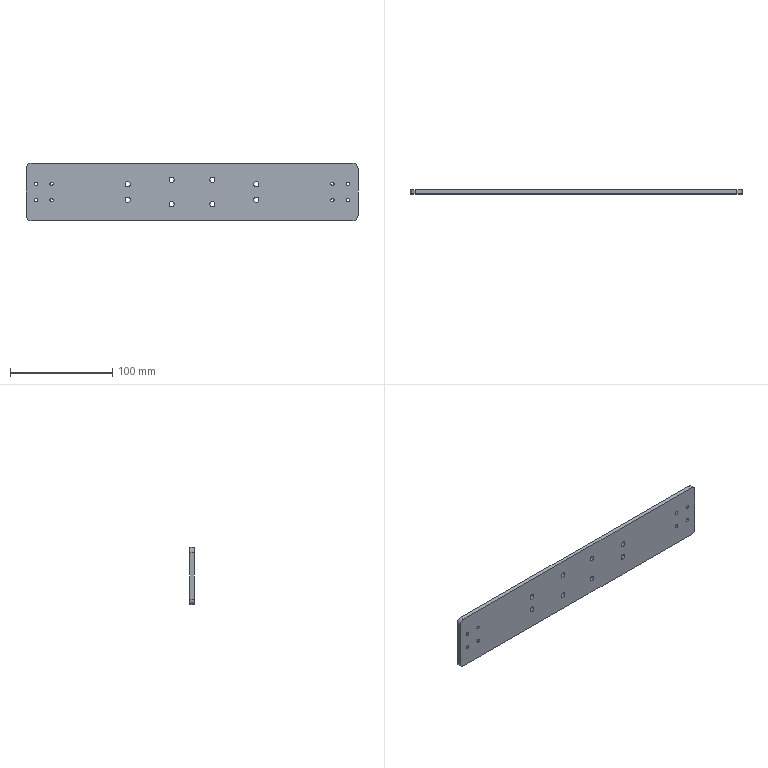Part | SolidWorks | features BaseBody 1 | 1 solid | 42 faces | box 325 x 4 x 56 mm | volume 71803 mm3 | cylinder 36 | plane 6 | commonest cylinder face diameters 3.2 x16 5 x8 5.2 x8 10 x4
STEP:
#1=CARTESIAN_POINT('',(63.,4.,10.1));
#2=VERTEX_POINT('',#1);
#3=CARTESIAN_POINT('',(63.,4.,4.9));
#4=VERTEX_POINT('',#3);
#5=CARTESIAN_POINT('',(63.,4.,7.5));
#6=DIRECTION('',(0.,-1.,0.));
#7=DIRECTION('',(0.,0.,-1.));
#8=AXIS2_PLACEMENT_3D('',#5,#6,#7);
#9=CIRCLE('',#8,2.6);
#10=EDGE_CURVE('',#2,#4,#9,.T.);
#11=ORIENTED_EDGE('',*,*,#10,.F.);
#12=CARTESIAN_POINT('',(63.,0.,10.1));
#13=VERTEX_POINT('',#12);
#14=CARTESIAN_POINT('',(63.,4.,10.1));
#15=DIRECTION('',(0.,-1.,0.));
#16=VECTOR('',#15,1000.);
#17=LINE('',#14,#16);
#18=EDGE_CURVE('',#2,#13,#17,.T.);
#19=ORIENTED_EDGE('',*,*,#18,.T.);
#20=CARTESIAN_POINT('',(63.,0.,4.9));
#21=VERTEX_POINT('',#20);
#22=CARTESIAN_POINT('',(63.,0.,7.5));
#23=DIRECTION('',(0.,-1.,0.));
#24=DIRECTION('',(0.,0.,-1.));
#25=AXIS2_PLACEMENT_3D('',#22,#23,#24);
#26=CIRCLE('',#25,2.6);
#27=EDGE_CURVE('',#13,#21,#26,.T.);
#28=ORIENTED_EDGE('',*,*,#27,.T.);
#29=CARTESIAN_POINT('',(63.,4.,4.9));
#30=DIRECTION('',(0.,-1.,0.));
#31=VECTOR('',#30,1000.);
#32=LINE('',#29,#31);
#33=EDGE_CURVE('',#4,#21,#32,.T.);
#34=ORIENTED_EDGE('',*,*,#33,.F.);
#35=EDGE_LOOP('',(#11,#19,#28,#34));
#36=FACE_OUTER_BOUND('',#35,.T.);
#37=CARTESIAN_POINT('',(63.,4.,7.5));
#38=DIRECTION('',(0.,-1.,0.));
#39=DIRECTION('',(0.,0.,-1.));
#40=AXIS2_PLACEMENT_3D('',#37,#38,#39);
#41=CYLINDRICAL_SURFACE('',#40,2.6);
#42=ADVANCED_FACE('',(#36),#41,.F.);
#43=CARTESIAN_POINT('',(63.,4.,-4.9));
#44=VERTEX_POINT('',#43);
#45=CARTESIAN_POINT('',(63.,4.,-10.1));
#46=VERTEX_POINT('',#45);
#47=CARTESIAN_POINT('',(63.,4.,-7.5));
#48=DIRECTION('',(0.,-1.,0.));
#49=DIRECTION('',(0.,0.,-1.));
#50=AXIS2_PLACEMENT_3D('',#47,#48,#49);
#51=CIRCLE('',#50,2.6);
#52=EDGE_CURVE('',#44,#46,#51,.T.);
#53=ORIENTED_EDGE('',*,*,#52,.F.);
#54=CARTESIAN_POINT('',(63.,0.,-4.9));
#55=VERTEX_POINT('',#54);
#56=CARTESIAN_POINT('',(63.,4.,-4.9));
#57=DIRECTION('',(0.,-1.,0.));
#58=VECTOR('',#57,1000.);
#59=LINE('',#56,#58);
#60=EDGE_CURVE('',#44,#55,#59,.T.);
#61=ORIENTED_EDGE('',*,*,#60,.T.);
#62=CARTESIAN_POINT('',(63.,0.,-10.1));
#63=VERTEX_POINT('',#62);
#64=CARTESIAN_POINT('',(63.,0.,-7.5));
#65=DIRECTION('',(0.,-1.,0.));
#66=DIRECTION('',(0.,0.,-1.));
#67=AXIS2_PLACEMENT_3D('',#64,#65,#66);
#68=CIRCLE('',#67,2.6);
#69=EDGE_CURVE('',#55,#63,#68,.T.);
#70=ORIENTED_EDGE('',*,*,#69,.T.);
#71=CARTESIAN_POINT('',(63.,4.,-10.1));
#72=DIRECTION('',(0.,-1.,0.));
#73=VECTOR('',#72,1000.);
#74=LINE('',#71,#73);
#75=EDGE_CURVE('',#46,#63,#74,.T.);
#76=ORIENTED_EDGE('',*,*,#75,.F.);
#77=EDGE_LOOP('',(#53,#61,#70,#76));
#78=FACE_OUTER_BOUND('',#77,.T.);
#79=CARTESIAN_POINT('',(63.,4.,-7.5));
#80=DIRECTION('',(0.,-1.,0.));
#81=DIRECTION('',(0.,0.,-1.));
#82=AXIS2_PLACEMENT_3D('',#79,#80,#81);
#83=CYLINDRICAL_SURFACE('',#82,2.6);
#84=ADVANCED_FACE('',(#78),#83,.F.);
#85=CARTESIAN_POINT('',(-63.,4.,-4.9));
#86=VERTEX_POINT('',#85);
#87=CARTESIAN_POINT('',(-63.,4.,-10.1));
#88=VERTEX_POINT('',#87);
#89=CARTESIAN_POINT('',(-63.,4.,-7.5));
#90=DIRECTION('',(0.,-1.,0.));
#91=DIRECTION('',(0.,0.,-1.));
#92=AXIS2_PLACEMENT_3D('',#89,#90,#91);
#93=CIRCLE('',#92,2.6);
#94=EDGE_CURVE('',#86,#88,#93,.T.);
#95=ORIENTED_EDGE('',*,*,#94,.F.);
#96=CARTESIAN_POINT('',(-63.,0.,-4.9));
#97=VERTEX_POINT('',#96);
#98=CARTESIAN_POINT('',(-63.,4.,-4.9));
#99=DIRECTION('',(0.,-1.,0.));
#100=VECTOR('',#99,1000.);
#101=LINE('',#98,#100);
#102=EDGE_CURVE('',#86,#97,#101,.T.);
#103=ORIENTED_EDGE('',*,*,#102,.T.);
#104=CARTESIAN_POINT('',(-63.,0.,-10.1));
#105=VERTEX_POINT('',#104);
#106=CARTESIAN_POINT('',(-63.,0.,-7.5));
#107=DIRECTION('',(0.,-1.,0.));
#108=DIRECTION('',(0.,0.,-1.));
#109=AXIS2_PLACEMENT_3D('',#106,#107,#108);
#110=CIRCLE('',#109,2.6);
#111=EDGE_CURVE('',#97,#105,#110,.T.);
#112=ORIENTED_EDGE('',*,*,#111,.T.);
#113=CARTESIAN_POINT('',(-63.,4.,-10.1));
#114=DIRECTION('',(0.,-1.,0.));
#115=VECTOR('',#114,1000.);
#116=LINE('',#113,#115);
#117=EDGE_CURVE('',#88,#105,#116,.T.);
#118=ORIENTED_EDGE('',*,*,#117,.F.);
#119=EDGE_LOOP('',(#95,#103,#112,#118));
#120=FACE_OUTER_BOUND('',#119,.T.);
#121=CARTESIAN_POINT('',(-63.,4.,-7.5));
#122=DIRECTION('',(0.,-1.,0.));
#123=DIRECTION('',(0.,0.,-1.));
#124=AXIS2_PLACEMENT_3D('',#121,#122,#123);
#125=CYLINDRICAL_SURFACE('',#124,2.6);
#126=ADVANCED_FACE('',(#120),#125,.F.);
#127=CARTESIAN_POINT('',(-63.,4.,10.1));
#128=VERTEX_POINT('',#127);
#129=CARTESIAN_POINT('',(-63.,4.,4.9));
#130=VERTEX_POINT('',#129);
#131=CARTESIAN_POINT('',(-63.,4.,7.5));
#132=DIRECTION('',(0.,-1.,0.));
#133=DIRECTION('',(0.,0.,-1.));
#134=AXIS2_PLACEMENT_3D('',#131,#132,#133);
#135=CIRCLE('',#134,2.6);
#136=EDGE_CURVE('',#128,#130,#135,.T.);
#137=ORIENTED_EDGE('',*,*,#136,.F.);
#138=CARTESIAN_POINT('',(-63.,0.,10.1));
#139=VERTEX_POINT('',#138);
#140=CARTESIAN_POINT('',(-63.,4.,10.1));
#141=DIRECTION('',(0.,-1.,0.));
#142=VECTOR('',#141,1000.);
#143=LINE('',#140,#142);
#144=EDGE_CURVE('',#128,#139,#143,.T.);
#145=ORIENTED_EDGE('',*,*,#144,.T.);
#146=CARTESIAN_POINT('',(-63.,0.,4.9));
#147=VERTEX_POINT('',#146);
#148=CARTESIAN_POINT('',(-63.,0.,7.5));
#149=DIRECTION('',(0.,-1.,0.));
#150=DIRECTION('',(0.,0.,-1.));
#151=AXIS2_PLACEMENT_3D('',#148,#149,#150);
#152=CIRCLE('',#151,2.6);
#153=EDGE_CURVE('',#139,#147,#152,.T.);
#154=ORIENTED_EDGE('',*,*,#153,.T.);
#155=CARTESIAN_POINT('',(-63.,4.,4.9));
#156=DIRECTION('',(0.,-1.,0.));
#157=VECTOR('',#156,1000.);
#158=LINE('',#155,#157);
#159=EDGE_CURVE('',#130,#147,#158,.T.);
#160=ORIENTED_EDGE('',*,*,#159,.F.);
#161=EDGE_LOOP('',(#137,#145,#154,#160));
#162=FACE_OUTER_BOUND('',#161,.T.);
#163=CARTESIAN_POINT('',(-63.,4.,7.5));
#164=DIRECTION('',(0.,-1.,0.));
#165=DIRECTION('',(0.,0.,-1.));
#166=AXIS2_PLACEMENT_3D('',#163,#164,#165);
#167=CYLINDRICAL_SURFACE('',#166,2.6);
#168=ADVANCED_FACE('',(#162),#167,.F.);
#169=CARTESIAN_POINT('',(152.5,4.,-6.4));
#170=VERTEX_POINT('',#169);
#171=CARTESIAN_POINT('',(152.5,4.,-9.6));
#172=VERTEX_POINT('',#171);
#173=CARTESIAN_POINT('',(152.5,4.,-8.));
#174=DIRECTION('',(0.,-1.,0.));
#175=DIRECTION('',(0.,0.,-1.));
#176=AXIS2_PLACEMENT_3D('',#173,#174,#175);
#177=CIRCLE('',#176,1.6);
#178=EDGE_CURVE('',#170,#172,#177,.T.);
#179=ORIENTED_EDGE('',*,*,#178,.F.);
#180=CARTESIAN_POINT('',(152.5,0.,-6.4));
#181=VERTEX_POINT('',#180);
#182=CARTESIAN_POINT('',(152.5,4.,-6.4));
#183=DIRECTION('',(0.,-1.,0.));
#184=VECTOR('',#183,1000.);
#185=LINE('',#182,#184);
#186=EDGE_CURVE('',#170,#181,#185,.T.);
#187=ORIENTED_EDGE('',*,*,#186,.T.);
#188=CARTESIAN_POINT('',(152.5,0.,-9.6));
#189=VERTEX_POINT('',#188);
#190=CARTESIAN_POINT('',(152.5,0.,-8.));
#191=DIRECTION('',(0.,-1.,0.));
#192=DIRECTION('',(0.,0.,-1.));
#193=AXIS2_PLACEMENT_3D('',#190,#191,#192);
#194=CIRCLE('',#193,1.6);
#195=EDGE_CURVE('',#181,#189,#194,.T.);
#196=ORIENTED_EDGE('',*,*,#195,.T.);
#197=CARTESIAN_POINT('',(152.5,4.,-9.6));
#198=DIRECTION('',(0.,-1.,0.));
#199=VECTOR('',#198,1000.);
#200=LINE('',#197,#199);
#201=EDGE_CURVE('',#172,#189,#200,.T.);
#202=ORIENTED_EDGE('',*,*,#201,.F.);
#203=EDGE_LOOP('',(#179,#187,#196,#202));
#204=FACE_OUTER_BOUND('',#203,.T.);
#205=CARTESIAN_POINT('',(152.5,4.,-8.));
#206=DIRECTION('',(0.,-1.,0.));
#207=DIRECTION('',(0.,0.,-1.));
#208=AXIS2_PLACEMENT_3D('',#205,#206,#207);
#209=CYLINDRICAL_SURFACE('',#208,1.6);
#210=ADVANCED_FACE('',(#204),#209,.F.);
#211=CARTESIAN_POINT('',(137.5,4.,-6.4));
#212=VERTEX_POINT('',#211);
#213=CARTESIAN_POINT('',(137.5,4.,-9.6));
#214=VERTEX_POINT('',#213);
#215=CARTESIAN_POINT('',(137.5,4.,-8.));
#216=DIRECTION('',(0.,-1.,0.));
#217=DIRECTION('',(0.,0.,-1.));
#218=AXIS2_PLACEMENT_3D('',#215,#216,#217);
#219=CIRCLE('',#218,1.6);
#220=EDGE_CURVE('',#212,#214,#219,.T.);
#221=ORIENTED_EDGE('',*,*,#220,.F.);
#222=CARTESIAN_POINT('',(137.5,0.,-6.4));
#223=VERTEX_POINT('',#222);
#224=CARTESIAN_POINT('',(137.5,4.,-6.4));
#225=DIRECTION('',(0.,-1.,0.));
#226=VECTOR('',#225,1000.);
#227=LINE('',#224,#226);
#228=EDGE_CURVE('',#212,#223,#227,.T.);
#229=ORIENTED_EDGE('',*,*,#228,.T.);
#230=CARTESIAN_POINT('',(137.5,0.,-9.6));
#231=VERTEX_POINT('',#230);
#232=CARTESIAN_POINT('',(137.5,0.,-8.));
#233=DIRECTION('',(0.,-1.,0.));
#234=DIRECTION('',(0.,0.,-1.));
#235=AXIS2_PLACEMENT_3D('',#232,#233,#234);
#236=CIRCLE('',#235,1.6);
#237=EDGE_CURVE('',#223,#231,#236,.T.);
#238=ORIENTED_EDGE('',*,*,#237,.T.);
#239=CARTESIAN_POINT('',(137.5,4.,-9.6));
#240=DIRECTION('',(0.,-1.,0.));
#241=VECTOR('',#240,1000.);
#242=LINE('',#239,#241);
#243=EDGE_CURVE('',#214,#231,#242,.T.);
#244=ORIENTED_EDGE('',*,*,#243,.F.);
#245=EDGE_LOOP('',(#221,#229,#238,#244));
#246=FACE_OUTER_BOUND('',#245,.T.);
#247=CARTESIAN_POINT('',(137.5,4.,-8.));
#248=DIRECTION('',(0.,-1.,0.));
#249=DIRECTION('',(0.,0.,-1.));
#250=AXIS2_PLACEMENT_3D('',#247,#248,#249);
#251=CYLINDRICAL_SURFACE('',#250,1.6);
#252=ADVANCED_FACE('',(#246),#251,.F.);
#253=CARTESIAN_POINT('',(152.5,4.,9.6));
#254=VERTEX_POINT('',#253);
#255=CARTESIAN_POINT('',(152.5,4.,6.4));
#256=VERTEX_POINT('',#255);
#257=CARTESIAN_POINT('',(152.5,4.,8.));
#258=DIRECTION('',(0.,-1.,0.));
#259=DIRECTION('',(0.,0.,-1.));
#260=AXIS2_PLACEMENT_3D('',#257,#258,#259);
#261=CIRCLE('',#260,1.6);
#262=EDGE_CURVE('',#254,#256,#261,.T.);
#263=ORIENTED_EDGE('',*,*,#262,.F.);
#264=CARTESIAN_POINT('',(152.5,0.,9.6));
#265=VERTEX_POINT('',#264);
#266=CARTESIAN_POINT('',(152.5,4.,9.6));
#267=DIRECTION('',(0.,-1.,0.));
#268=VECTOR('',#267,1000.);
#269=LINE('',#266,#268);
#270=EDGE_CURVE('',#254,#265,#269,.T.);
#271=ORIENTED_EDGE('',*,*,#270,.T.);
#272=CARTESIAN_POINT('',(152.5,0.,6.4));
#273=VERTEX_POINT('',#272);
#274=CARTESIAN_POINT('',(152.5,0.,8.));
#275=DIRECTION('',(0.,-1.,0.));
#276=DIRECTION('',(0.,0.,-1.));
#277=AXIS2_PLACEMENT_3D('',#274,#275,#276);
#278=CIRCLE('',#277,1.6);
#279=EDGE_CURVE('',#265,#273,#278,.T.);
#280=ORIENTED_EDGE('',*,*,#279,.T.);
#281=CARTESIAN_POINT('',(152.5,4.,6.4));
#282=DIRECTION('',(0.,-1.,0.));
#283=VECTOR('',#282,1000.);
#284=LINE('',#281,#283);
#285=EDGE_CURVE('',#256,#273,#284,.T.);
#286=ORIENTED_EDGE('',*,*,#285,.F.);
#287=EDGE_LOOP('',(#263,#271,#280,#286));
#288=FACE_OUTER_BOUND('',#287,.T.);
#289=CARTESIAN_POINT('',(152.5,4.,8.));
#290=DIRECTION('',(0.,-1.,0.));
#291=DIRECTION('',(0.,0.,-1.));
#292=AXIS2_PLACEMENT_3D('',#289,#290,#291);
#293=CYLINDRICAL_SURFACE('',#292,1.6);
#294=ADVANCED_FACE('',(#288),#293,.F.);
#295=CARTESIAN_POINT('',(137.5,4.,9.6));
#296=VERTEX_POINT('',#295);
#297=CARTESIAN_POINT('',(137.5,4.,6.4));
#298=VERTEX_POINT('',#297);
#299=CARTESIAN_POINT('',(137.5,4.,8.));
#300=DIRECTION('',(0.,-1.,0.));
#301=DIRECTION('',(0.,0.,-1.));
#302=AXIS2_PLACEMENT_3D('',#299,#300,#301);
#303=CIRCLE('',#302,1.6);
#304=EDGE_CURVE('',#296,#298,#303,.T.);
#305=ORIENTED_EDGE('',*,*,#304,.F.);
#306=CARTESIAN_POINT('',(137.5,0.,9.6));
#307=VERTEX_POINT('',#306);
#308=CARTESIAN_POINT('',(137.5,4.,9.6));
#309=DIRECTION('',(0.,-1.,0.));
#310=VECTOR('',#309,1000.);
#311=LINE('',#308,#310);
#312=EDGE_CURVE('',#296,#307,#311,.T.);
#313=ORIENTED_EDGE('',*,*,#312,.T.);
#314=CARTESIAN_POINT('',(137.5,0.,6.4));
#315=VERTEX_POINT('',#314);
#316=CARTESIAN_POINT('',(137.5,0.,8.));
#317=DIRECTION('',(0.,-1.,0.));
#318=DIRECTION('',(0.,0.,-1.));
#319=AXIS2_PLACEMENT_3D('',#316,#317,#318);
#320=CIRCLE('',#319,1.6);
#321=EDGE_CURVE('',#307,#315,#320,.T.);
#322=ORIENTED_EDGE('',*,*,#321,.T.);
#323=CARTESIAN_POINT('',(137.5,4.,6.4));
#324=DIRECTION('',(0.,-1.,0.));
#325=VECTOR('',#324,1000.);
#326=LINE('',#323,#325);
#327=EDGE_CURVE('',#298,#315,#326,.T.);
#328=ORIENTED_EDGE('',*,*,#327,.F.);
#329=EDGE_LOOP('',(#305,#313,#322,#328));
#330=FACE_OUTER_BOUND('',#329,.T.);
#331=CARTESIAN_POINT('',(137.5,4.,8.));
#332=DIRECTION('',(0.,-1.,0.));
#333=DIRECTION('',(0.,0.,-1.));
#334=AXIS2_PLACEMENT_3D('',#331,#332,#333);
#335=CYLINDRICAL_SURFACE('',#334,1.6);
#336=ADVANCED_FACE('',(#330),#335,.F.);
#337=CARTESIAN_POINT('',(20.,4.,-9.5));
#338=VERTEX_POINT('',#337);
#339=CARTESIAN_POINT('',(20.,4.,-14.5));
#340=VERTEX_POINT('',#339);
#341=CARTESIAN_POINT('',(20.,4.,-12.));
#342=DIRECTION('',(0.,-1.,0.));
#343=DIRECTION('',(0.,0.,-1.));
#344=AXIS2_PLACEMENT_3D('',#341,#342,#343);
#345=CIRCLE('',#344,2.5);
#346=EDGE_CURVE('',#338,#340,#345,.T.);
#347=ORIENTED_EDGE('',*,*,#346,.F.);
#348=CARTESIAN_POINT('',(20.,0.,-9.5));
#349=VERTEX_POINT('',#348);
#350=CARTESIAN_POINT('',(20.,4.,-9.5));
#351=DIRECTION('',(0.,-1.,0.));
#352=VECTOR('',#351,1000.);
#353=LINE('',#350,#352);
#354=EDGE_CURVE('',#338,#349,#353,.T.);
#355=ORIENTED_EDGE('',*,*,#354,.T.);
#356=CARTESIAN_POINT('',(20.,0.,-14.5));
#357=VERTEX_POINT('',#356);
#358=CARTESIAN_POINT('',(20.,0.,-12.));
#359=DIRECTION('',(0.,-1.,0.));
#360=DIRECTION('',(0.,0.,-1.));
#361=AXIS2_PLACEMENT_3D('',#358,#359,#360);
#362=CIRCLE('',#361,2.5);
#363=EDGE_CURVE('',#349,#357,#362,.T.);
#364=ORIENTED_EDGE('',*,*,#363,.T.);
#365=CARTESIAN_POINT('',(20.,4.,-14.5));
#366=DIRECTION('',(0.,-1.,0.));
#367=VECTOR('',#366,1000.);
#368=LINE('',#365,#367);
#369=EDGE_CURVE('',#340,#357,#368,.T.);
#370=ORIENTED_EDGE('',*,*,#369,.F.);
#371=EDGE_LOOP('',(#347,#355,#364,#370));
#372=FACE_OUTER_BOUND('',#371,.T.);
#373=CARTESIAN_POINT('',(20.,4.,-12.));
#374=DIRECTION('',(0.,-1.,0.));
#375=DIRECTION('',(0.,0.,-1.));
#376=AXIS2_PLACEMENT_3D('',#373,#374,#375);
#377=CYLINDRICAL_SURFACE('',#376,2.5);
#378=ADVANCED_FACE('',(#372),#377,.F.);
#379=CARTESIAN_POINT('',(20.,4.,14.5));
#380=VERTEX_POINT('',#379);
#381=CARTESIAN_POINT('',(20.,4.,9.5));
#382=VERTEX_POINT('',#381);
#383=CARTESIAN_POINT('',(20.,4.,12.));
#384=DIRECTION('',(0.,-1.,0.));
#385=DIRECTION('',(0.,0.,-1.));
#386=AXIS2_PLACEMENT_3D('',#383,#384,#385);
#387=CIRCLE('',#386,2.5);
#388=EDGE_CURVE('',#380,#382,#387,.T.);
#389=ORIENTED_EDGE('',*,*,#388,.F.);
#390=CARTESIAN_POINT('',(20.,0.,14.5));
#391=VERTEX_POINT('',#390);
#392=CARTESIAN_POINT('',(20.,4.,14.5));
#393=DIRECTION('',(0.,-1.,0.));
#394=VECTOR('',#393,1000.);
#395=LINE('',#392,#394);
#396=EDGE_CURVE('',#380,#391,#395,.T.);
#397=ORIENTED_EDGE('',*,*,#396,.T.);
#398=CARTESIAN_POINT('',(20.,0.,9.5));
#399=VERTEX_POINT('',#398);
#400=CARTESIAN_POINT('',(20.,0.,12.));
#401=DIRECTION('',(0.,-1.,0.));
#402=DIRECTION('',(0.,0.,-1.));
#403=AXIS2_PLACEMENT_3D('',#400,#401,#402);
#404=CIRCLE('',#403,2.5);
#405=EDGE_CURVE('',#391,#399,#404,.T.);
#406=ORIENTED_EDGE('',*,*,#405,.T.);
#407=CARTESIAN_POINT('',(20.,4.,9.5));
#408=DIRECTION('',(0.,-1.,0.));
#409=VECTOR('',#408,1000.);
#410=LINE('',#407,#409);
#411=EDGE_CURVE('',#382,#399,#410,.T.);
#412=ORIENTED_EDGE('',*,*,#411,.F.);
#413=EDGE_LOOP('',(#389,#397,#406,#412));
#414=FACE_OUTER_BOUND('',#413,.T.);
#415=CARTESIAN_POINT('',(20.,4.,12.));
#416=DIRECTION('',(0.,-1.,0.));
#417=DIRECTION('',(0.,0.,-1.));
#418=AXIS2_PLACEMENT_3D('',#415,#416,#417);
#419=CYLINDRICAL_SURFACE('',#418,2.5);
#420=ADVANCED_FACE('',(#414),#419,.F.);
#421=CARTESIAN_POINT('',(-20.,4.,14.5));
#422=VERTEX_POINT('',#421);
#423=CARTESIAN_POINT('',(-20.,4.,9.5));
#424=VERTEX_POINT('',#423);
#425=CARTESIAN_POINT('',(-20.,4.,12.));
#426=DIRECTION('',(0.,-1.,0.));
#427=DIRECTION('',(0.,0.,-1.));
#428=AXIS2_PLACEMENT_3D('',#425,#426,#427);
#429=CIRCLE('',#428,2.5);
#430=EDGE_CURVE('',#422,#424,#429,.T.);
#431=ORIENTED_EDGE('',*,*,#430,.F.);
#432=CARTESIAN_POINT('',(-20.,0.,14.5));
#433=VERTEX_POINT('',#432);
#434=CARTESIAN_POINT('',(-20.,4.,14.5));
#435=DIRECTION('',(0.,-1.,0.));
#436=VECTOR('',#435,1000.);
#437=LINE('',#434,#436);
#438=EDGE_CURVE('',#422,#433,#437,.T.);
#439=ORIENTED_EDGE('',*,*,#438,.T.);
#440=CARTESIAN_POINT('',(-20.,0.,9.5));
#441=VERTEX_POINT('',#440);
#442=CARTESIAN_POINT('',(-20.,0.,12.));
#443=DIRECTION('',(0.,-1.,0.));
#444=DIRECTION('',(0.,0.,-1.));
#445=AXIS2_PLACEMENT_3D('',#442,#443,#444);
#446=CIRCLE('',#445,2.5);
#447=EDGE_CURVE('',#433,#441,#446,.T.);
#448=ORIENTED_EDGE('',*,*,#447,.T.);
#449=CARTESIAN_POINT('',(-20.,4.,9.5));
#450=DIRECTION('',(0.,-1.,0.));
#451=VECTOR('',#450,1000.);
#452=LINE('',#449,#451);
#453=EDGE_CURVE('',#424,#441,#452,.T.);
#454=ORIENTED_EDGE('',*,*,#453,.F.);
#455=EDGE_LOOP('',(#431,#439,#448,#454));
#456=FACE_OUTER_BOUND('',#455,.T.);
#457=CARTESIAN_POINT('',(-20.,4.,12.));
#458=DIRECTION('',(0.,-1.,0.));
#459=DIRECTION('',(0.,0.,-1.));
#460=AXIS2_PLACEMENT_3D('',#457,#458,#459);
#461=CYLINDRICAL_SURFACE('',#460,2.5);
#462=ADVANCED_FACE('',(#456),#461,.F.);
#463=CARTESIAN_POINT('',(-20.,4.,-9.5));
#464=VERTEX_POINT('',#463);
#465=CARTESIAN_POINT('',(-20.,4.,-14.5));
#466=VERTEX_POINT('',#465);
#467=CARTESIAN_POINT('',(-20.,4.,-12.));
#468=DIRECTION('',(0.,-1.,0.));
#469=DIRECTION('',(0.,0.,-1.));
#470=AXIS2_PLACEMENT_3D('',#467,#468,#469);
#471=CIRCLE('',#470,2.5);
#472=EDGE_CURVE('',#464,#466,#471,.T.);
#473=ORIENTED_EDGE('',*,*,#472,.F.);
#474=CARTESIAN_POINT('',(-20.,0.,-9.5));
#475=VERTEX_POINT('',#474);
#476=CARTESIAN_POINT('',(-20.,4.,-9.5));
#477=DIRECTION('',(0.,-1.,0.));
#478=VECTOR('',#477,1000.);
#479=LINE('',#476,#478);
#480=EDGE_CURVE('',#464,#475,#479,.T.);
#481=ORIENTED_EDGE('',*,*,#480,.T.);
#482=CARTESIAN_POINT('',(-20.,0.,-14.5));
#483=VERTEX_POINT('',#482);
#484=CARTESIAN_POINT('',(-20.,0.,-12.));
#485=DIRECTION('',(0.,-1.,0.));
#486=DIRECTION('',(0.,0.,-1.));
#487=AXIS2_PLACEMENT_3D('',#484,#485,#486);
#488=CIRCLE('',#487,2.5);
#489=EDGE_CURVE('',#475,#483,#488,.T.);
#490=ORIENTED_EDGE('',*,*,#489,.T.);
#491=CARTESIAN_POINT('',(-20.,4.,-14.5));
#492=DIRECTION('',(0.,-1.,0.));
#493=VECTOR('',#492,1000.);
#494=LINE('',#491,#493);
#495=EDGE_CURVE('',#466,#483,#494,.T.);
#496=ORIENTED_EDGE('',*,*,#495,.F.);
#497=EDGE_LOOP('',(#473,#481,#490,#496));
#498=FACE_OUTER_BOUND('',#497,.T.);
#499=CARTESIAN_POINT('',(-20.,4.,-12.));
#500=DIRECTION('',(0.,-1.,0.));
#501=DIRECTION('',(0.,0.,-1.));
#502=AXIS2_PLACEMENT_3D('',#499,#500,#501);
#503=CYLINDRICAL_SURFACE('',#502,2.5);
#504=ADVANCED_FACE('',(#498),#503,.F.);
#505=CARTESIAN_POINT('',(-137.5,4.,9.6));
#506=VERTEX_POINT('',#505);
#507=CARTESIAN_POINT('',(-137.5,4.,6.4));
#508=VERTEX_POINT('',#507);
#509=CARTESIAN_POINT('',(-137.5,4.,8.));
#510=DIRECTION('',(0.,-1.,0.));
#511=DIRECTION('',(0.,0.,-1.));
#512=AXIS2_PLACEMENT_3D('',#509,#510,#511);
#513=CIRCLE('',#512,1.6);
#514=EDGE_CURVE('',#506,#508,#513,.T.);
#515=ORIENTED_EDGE('',*,*,#514,.F.);
#516=CARTESIAN_POINT('',(-137.5,0.,9.6));
#517=VERTEX_POINT('',#516);
#518=CARTESIAN_POINT('',(-137.5,4.,9.6));
#519=DIRECTION('',(0.,-1.,0.));
#520=VECTOR('',#519,1000.);
#521=LINE('',#518,#520);
#522=EDGE_CURVE('',#506,#517,#521,.T.);
#523=ORIENTED_EDGE('',*,*,#522,.T.);
#524=CARTESIAN_POINT('',(-137.5,0.,6.4));
#525=VERTEX_POINT('',#524);
#526=CARTESIAN_POINT('',(-137.5,0.,8.));
#527=DIRECTION('',(0.,-1.,0.));
#528=DIRECTION('',(0.,0.,-1.));
#529=AXIS2_PLACEMENT_3D('',#526,#527,#528);
#530=CIRCLE('',#529,1.6);
#531=EDGE_CURVE('',#517,#525,#530,.T.);
#532=ORIENTED_EDGE('',*,*,#531,.T.);
#533=CARTESIAN_POINT('',(-137.5,4.,6.4));
#534=DIRECTION('',(0.,-1.,0.));
#535=VECTOR('',#534,1000.);
#536=LINE('',#533,#535);
#537=EDGE_CURVE('',#508,#525,#536,.T.);
#538=ORIENTED_EDGE('',*,*,#537,.F.);
#539=EDGE_LOOP('',(#515,#523,#532,#538));
#540=FACE_OUTER_BOUND('',#539,.T.);
#541=CARTESIAN_POINT('',(-137.5,4.,8.));
#542=DIRECTION('',(0.,-1.,0.));
#543=DIRECTION('',(0.,0.,-1.));
#544=AXIS2_PLACEMENT_3D('',#541,#542,#543);
#545=CYLINDRICAL_SURFACE('',#544,1.6);
#546=ADVANCED_FACE('',(#540),#545,.F.);
#547=CARTESIAN_POINT('',(-152.5,4.,9.6));
#548=VERTEX_POINT('',#547);
#549=CARTESIAN_POINT('',(-152.5,4.,6.4));
#550=VERTEX_POINT('',#549);
#551=CARTESIAN_POINT('',(-152.5,4.,8.));
#552=DIRECTION('',(0.,-1.,0.));
#553=DIRECTION('',(0.,0.,-1.));
#554=AXIS2_PLACEMENT_3D('',#551,#552,#553);
#555=CIRCLE('',#554,1.6);
#556=EDGE_CURVE('',#548,#550,#555,.T.);
#557=ORIENTED_EDGE('',*,*,#556,.F.);
#558=CARTESIAN_POINT('',(-152.5,0.,9.6));
#559=VERTEX_POINT('',#558);
#560=CARTESIAN_POINT('',(-152.5,4.,9.6));
#561=DIRECTION('',(0.,-1.,0.));
#562=VECTOR('',#561,1000.);
#563=LINE('',#560,#562);
#564=EDGE_CURVE('',#548,#559,#563,.T.);
#565=ORIENTED_EDGE('',*,*,#564,.T.);
#566=CARTESIAN_POINT('',(-152.5,0.,6.4));
#567=VERTEX_POINT('',#566);
#568=CARTESIAN_POINT('',(-152.5,0.,8.));
#569=DIRECTION('',(0.,-1.,0.));
#570=DIRECTION('',(0.,0.,-1.));
#571=AXIS2_PLACEMENT_3D('',#568,#569,#570);
#572=CIRCLE('',#571,1.6);
#573=EDGE_CURVE('',#559,#567,#572,.T.);
#574=ORIENTED_EDGE('',*,*,#573,.T.);
#575=CARTESIAN_POINT('',(-152.5,4.,6.4));
#576=DIRECTION('',(0.,-1.,0.));
#577=VECTOR('',#576,1000.);
#578=LINE('',#575,#577);
#579=EDGE_CURVE('',#550,#567,#578,.T.);
#580=ORIENTED_EDGE('',*,*,#579,.F.);
#581=EDGE_LOOP('',(#557,#565,#574,#580));
#582=FACE_OUTER_BOUND('',#581,.T.);
#583=CARTESIAN_POINT('',(-152.5,4.,8.));
#584=DIRECTION('',(0.,-1.,0.));
#585=DIRECTION('',(0.,0.,-1.));
#586=AXIS2_PLACEMENT_3D('',#583,#584,#585);
#587=CYLINDRICAL_SURFACE('',#586,1.6);
#588=ADVANCED_FACE('',(#582),#587,.F.);
#589=CARTESIAN_POINT('',(-137.5,4.,-6.4));
#590=VERTEX_POINT('',#589);
#591=CARTESIAN_POINT('',(-137.5,4.,-9.6));
#592=VERTEX_POINT('',#591);
#593=CARTESIAN_POINT('',(-137.5,4.,-8.));
#594=DIRECTION('',(0.,-1.,0.));
#595=DIRECTION('',(0.,0.,-1.));
#596=AXIS2_PLACEMENT_3D('',#593,#594,#595);
#597=CIRCLE('',#596,1.6);
#598=EDGE_CURVE('',#590,#592,#597,.T.);
#599=ORIENTED_EDGE('',*,*,#598,.F.);
#600=CARTESIAN_POINT('',(-137.5,0.,-6.4));
#601=VERTEX_POINT('',#600);
#602=CARTESIAN_POINT('',(-137.5,4.,-6.4));
#603=DIRECTION('',(0.,-1.,0.));
#604=VECTOR('',#603,1000.);
#605=LINE('',#602,#604);
#606=EDGE_CURVE('',#590,#601,#605,.T.);
#607=ORIENTED_EDGE('',*,*,#606,.T.);
#608=CARTESIAN_POINT('',(-137.5,0.,-9.6));
#609=VERTEX_POINT('',#608);
#610=CARTESIAN_POINT('',(-137.5,0.,-8.));
#611=DIRECTION('',(0.,-1.,0.));
#612=DIRECTION('',(0.,0.,-1.));
#613=AXIS2_PLACEMENT_3D('',#610,#611,#612);
#614=CIRCLE('',#613,1.6);
#615=EDGE_CURVE('',#601,#609,#614,.T.);
#616=ORIENTED_EDGE('',*,*,#615,.T.);
#617=CARTESIAN_POINT('',(-137.5,4.,-9.6));
#618=DIRECTION('',(0.,-1.,0.));
#619=VECTOR('',#618,1000.);
#620=LINE('',#617,#619);
#621=EDGE_CURVE('',#592,#609,#620,.T.);
#622=ORIENTED_EDGE('',*,*,#621,.F.);
#623=EDGE_LOOP('',(#599,#607,#616,#622));
#624=FACE_OUTER_BOUND('',#623,.T.);
#625=CARTESIAN_POINT('',(-137.5,4.,-8.));
#626=DIRECTION('',(0.,-1.,0.));
#627=DIRECTION('',(0.,0.,-1.));
#628=AXIS2_PLACEMENT_3D('',#625,#626,#627);
#629=CYLINDRICAL_SURFACE('',#628,1.6);
#630=ADVANCED_FACE('',(#624),#629,.F.);
#631=CARTESIAN_POINT('',(-152.5,4.,-6.4));
#632=VERTEX_POINT('',#631);
#633=CARTESIAN_POINT('',(-152.5,4.,-9.6));
#634=VERTEX_POINT('',#633);
#635=CARTESIAN_POINT('',(-152.5,4.,-8.));
#636=DIRECTION('',(0.,-1.,0.));
#637=DIRECTION('',(0.,0.,-1.));
#638=AXIS2_PLACEMENT_3D('',#635,#636,#637);
#639=CIRCLE('',#638,1.6);
#640=EDGE_CURVE('',#632,#634,#639,.T.);
#641=ORIENTED_EDGE('',*,*,#640,.F.);
#642=CARTESIAN_POINT('',(-152.5,0.,-6.4));
#643=VERTEX_POINT('',#642);
#644=CARTESIAN_POINT('',(-152.5,4.,-6.4));
#645=DIRECTION('',(0.,-1.,0.));
#646=VECTOR('',#645,1000.);
#647=LINE('',#644,#646);
#648=EDGE_CURVE('',#632,#643,#647,.T.);
#649=ORIENTED_EDGE('',*,*,#648,.T.);
#650=CARTESIAN_POINT('',(-152.5,0.,-9.6));
#651=VERTEX_POINT('',#650);
#652=CARTESIAN_POINT('',(-152.5,0.,-8.));
#653=DIRECTION('',(0.,-1.,0.));
#654=DIRECTION('',(0.,0.,-1.));
#655=AXIS2_PLACEMENT_3D('',#652,#653,#654);
#656=CIRCLE('',#655,1.6);
#657=EDGE_CURVE('',#643,#651,#656,.T.);
#658=ORIENTED_EDGE('',*,*,#657,.T.);
#659=CARTESIAN_POINT('',(-152.5,4.,-9.6));
#660=DIRECTION('',(0.,-1.,0.));
#661=VECTOR('',#660,1000.);
#662=LINE('',#659,#661);
#663=EDGE_CURVE('',#634,#651,#662,.T.);
#664=ORIENTED_EDGE('',*,*,#663,.F.);
#665=EDGE_LOOP('',(#641,#649,#658,#664));
#666=FACE_OUTER_BOUND('',#665,.T.);
#667=CARTESIAN_POINT('',(-152.5,4.,-8.));
#668=DIRECTION('',(0.,-1.,0.));
#669=DIRECTION('',(0.,0.,-1.));
#670=AXIS2_PLACEMENT_3D('',#667,#668,#669);
#671=CYLINDRICAL_SURFACE('',#670,1.6);
#672=ADVANCED_FACE('',(#666),#671,.F.);
#673=CARTESIAN_POINT('',(63.,0.,7.5));
#674=DIRECTION('',(0.,-1.,0.));
#675=DIRECTION('',(0.,0.,-1.));
#676=AXIS2_PLACEMENT_3D('',#673,#674,#675);
#677=CIRCLE('',#676,2.6);
#678=EDGE_CURVE('',#21,#13,#677,.T.);
#679=ORIENTED_EDGE('',*,*,#678,.F.);
#680=ORIENTED_EDGE('',*,*,#27,.F.);
#681=EDGE_LOOP('',(#679,#680));
#682=FACE_BOUND('',#681,.T.);
#683=CARTESIAN_POINT('',(63.,0.,-7.5));
#684=DIRECTION('',(0.,-1.,0.));
#685=DIRECTION('',(0.,0.,-1.));
#686=AXIS2_PLACEMENT_3D('',#683,#684,#685);
#687=CIRCLE('',#686,2.6);
#688=EDGE_CURVE('',#63,#55,#687,.T.);
#689=ORIENTED_EDGE('',*,*,#688,.F.);
#690=ORIENTED_EDGE('',*,*,#69,.F.);
#691=EDGE_LOOP('',(#689,#690));
#692=FACE_BOUND('',#691,.T.);
#693=CARTESIAN_POINT('',(-63.,0.,-7.5));
#694=DIRECTION('',(0.,-1.,0.));
#695=DIRECTION('',(0.,0.,-1.));
#696=AXIS2_PLACEMENT_3D('',#693,#694,#695);
#697=CIRCLE('',#696,2.6);
#698=EDGE_CURVE('',#105,#97,#697,.T.);
#699=ORIENTED_EDGE('',*,*,#698,.F.);
#700=ORIENTED_EDGE('',*,*,#111,.F.);
#701=EDGE_LOOP('',(#699,#700));
#702=FACE_BOUND('',#701,.T.);
#703=CARTESIAN_POINT('',(-63.,0.,7.5));
#704=DIRECTION('',(0.,-1.,0.));
#705=DIRECTION('',(0.,0.,-1.));
#706=AXIS2_PLACEMENT_3D('',#703,#704,#705);
#707=CIRCLE('',#706,2.6);
#708=EDGE_CURVE('',#147,#139,#707,.T.);
#709=ORIENTED_EDGE('',*,*,#708,.F.);
#710=ORIENTED_EDGE('',*,*,#153,.F.);
#711=EDGE_LOOP('',(#709,#710));
#712=FACE_BOUND('',#711,.T.);
#713=CARTESIAN_POINT('',(152.5,0.,-8.));
#714=DIRECTION('',(0.,-1.,0.));
#715=DIRECTION('',(0.,0.,-1.));
#716=AXIS2_PLACEMENT_3D('',#713,#714,#715);
#717=CIRCLE('',#716,1.6);
#718=EDGE_CURVE('',#189,#181,#717,.T.);
#719=ORIENTED_EDGE('',*,*,#718,.F.);
#720=ORIENTED_EDGE('',*,*,#195,.F.);
#721=EDGE_LOOP('',(#719,#720));
#722=FACE_BOUND('',#721,.T.);
#723=CARTESIAN_POINT('',(137.5,0.,-8.));
#724=DIRECTION('',(0.,-1.,0.));
#725=DIRECTION('',(0.,0.,-1.));
#726=AXIS2_PLACEMENT_3D('',#723,#724,#725);
#727=CIRCLE('',#726,1.6);
#728=EDGE_CURVE('',#231,#223,#727,.T.);
#729=ORIENTED_EDGE('',*,*,#728,.F.);
#730=ORIENTED_EDGE('',*,*,#237,.F.);
#731=EDGE_LOOP('',(#729,#730));
#732=FACE_BOUND('',#731,.T.);
#733=CARTESIAN_POINT('',(152.5,0.,8.));
#734=DIRECTION('',(0.,-1.,0.));
#735=DIRECTION('',(0.,0.,-1.));
#736=AXIS2_PLACEMENT_3D('',#733,#734,#735);
#737=CIRCLE('',#736,1.6);
#738=EDGE_CURVE('',#273,#265,#737,.T.);
#739=ORIENTED_EDGE('',*,*,#738,.F.);
#740=ORIENTED_EDGE('',*,*,#279,.F.);
#741=EDGE_LOOP('',(#739,#740));
#742=FACE_BOUND('',#741,.T.);
#743=CARTESIAN_POINT('',(137.5,0.,8.));
#744=DIRECTION('',(0.,-1.,0.));
#745=DIRECTION('',(0.,0.,-1.));
#746=AXIS2_PLACEMENT_3D('',#743,#744,#745);
#747=CIRCLE('',#746,1.6);
#748=EDGE_CURVE('',#315,#307,#747,.T.);
#749=ORIENTED_EDGE('',*,*,#748,.F.);
#750=ORIENTED_EDGE('',*,*,#321,.F.);
#751=EDGE_LOOP('',(#749,#750));
#752=FACE_BOUND('',#751,.T.);
#753=CARTESIAN_POINT('',(20.,0.,-12.));
#754=DIRECTION('',(0.,-1.,0.));
#755=DIRECTION('',(0.,0.,-1.));
#756=AXIS2_PLACEMENT_3D('',#753,#754,#755);
#757=CIRCLE('',#756,2.5);
#758=EDGE_CURVE('',#357,#349,#757,.T.);
#759=ORIENTED_EDGE('',*,*,#758,.F.);
#760=ORIENTED_EDGE('',*,*,#363,.F.);
#761=EDGE_LOOP('',(#759,#760));
#762=FACE_BOUND('',#761,.T.);
#763=CARTESIAN_POINT('',(20.,0.,12.));
#764=DIRECTION('',(0.,-1.,0.));
#765=DIRECTION('',(0.,0.,-1.));
#766=AXIS2_PLACEMENT_3D('',#763,#764,#765);
#767=CIRCLE('',#766,2.5);
#768=EDGE_CURVE('',#399,#391,#767,.T.);
#769=ORIENTED_EDGE('',*,*,#768,.F.);
#770=ORIENTED_EDGE('',*,*,#405,.F.);
#771=EDGE_LOOP('',(#769,#770));
#772=FACE_BOUND('',#771,.T.);
#773=CARTESIAN_POINT('',(-20.,0.,12.));
#774=DIRECTION('',(0.,-1.,0.));
#775=DIRECTION('',(0.,0.,-1.));
#776=AXIS2_PLACEMENT_3D('',#773,#774,#775);
#777=CIRCLE('',#776,2.5);
#778=EDGE_CURVE('',#441,#433,#777,.T.);
#779=ORIENTED_EDGE('',*,*,#778,.F.);
#780=ORIENTED_EDGE('',*,*,#447,.F.);
#781=EDGE_LOOP('',(#779,#780));
#782=FACE_BOUND('',#781,.T.);
#783=CARTESIAN_POINT('',(-20.,0.,-12.));
#784=DIRECTION('',(0.,-1.,0.));
#785=DIRECTION('',(0.,0.,-1.));
#786=AXIS2_PLACEMENT_3D('',#783,#784,#785);
#787=CIRCLE('',#786,2.5);
#788=EDGE_CURVE('',#483,#475,#787,.T.);
#789=ORIENTED_EDGE('',*,*,#788,.F.);
#790=ORIENTED_EDGE('',*,*,#489,.F.);
#791=EDGE_LOOP('',(#789,#790));
#792=FACE_BOUND('',#791,.T.);
#793=CARTESIAN_POINT('',(-137.5,0.,8.));
#794=DIRECTION('',(0.,-1.,0.));
#795=DIRECTION('',(0.,0.,-1.));
#796=AXIS2_PLACEMENT_3D('',#793,#794,#795);
#797=CIRCLE('',#796,1.6);
#798=EDGE_CURVE('',#525,#517,#797,.T.);
#799=ORIENTED_EDGE('',*,*,#798,.F.);
#800=ORIENTED_EDGE('',*,*,#531,.F.);
#801=EDGE_LOOP('',(#799,#800));
#802=FACE_BOUND('',#801,.T.);
#803=CARTESIAN_POINT('',(-152.5,0.,8.));
#804=DIRECTION('',(0.,-1.,0.));
#805=DIRECTION('',(0.,0.,-1.));
#806=AXIS2_PLACEMENT_3D('',#803,#804,#805);
#807=CIRCLE('',#806,1.6);
#808=EDGE_CURVE('',#567,#559,#807,.T.);
#809=ORIENTED_EDGE('',*,*,#808,.F.);
#810=ORIENTED_EDGE('',*,*,#573,.F.);
#811=EDGE_LOOP('',(#809,#810));
#812=FACE_BOUND('',#811,.T.);
#813=CARTESIAN_POINT('',(-137.5,0.,-8.));
#814=DIRECTION('',(0.,-1.,0.));
#815=DIRECTION('',(0.,0.,-1.));
#816=AXIS2_PLACEMENT_3D('',#813,#814,#815);
#817=CIRCLE('',#816,1.6);
#818=EDGE_CURVE('',#609,#601,#817,.T.);
#819=ORIENTED_EDGE('',*,*,#818,.F.);
#820=ORIENTED_EDGE('',*,*,#615,.F.);
#821=EDGE_LOOP('',(#819,#820));
#822=FACE_BOUND('',#821,.T.);
#823=CARTESIAN_POINT('',(-152.5,0.,-8.));
#824=DIRECTION('',(0.,-1.,0.));
#825=DIRECTION('',(0.,0.,-1.));
#826=AXIS2_PLACEMENT_3D('',#823,#824,#825);
#827=CIRCLE('',#826,1.6);
#828=EDGE_CURVE('',#651,#643,#827,.T.);
#829=ORIENTED_EDGE('',*,*,#828,.F.);
#830=ORIENTED_EDGE('',*,*,#657,.F.);
#831=EDGE_LOOP('',(#829,#830));
#832=FACE_BOUND('',#831,.T.);
#833=CARTESIAN_POINT('',(157.5,0.,28.));
#834=VERTEX_POINT('',#833);
#835=CARTESIAN_POINT('',(162.5,0.,23.));
#836=VERTEX_POINT('',#835);
#837=CARTESIAN_POINT('',(157.5,0.,23.));
#838=DIRECTION('',(0.,1.,0.));
#839=DIRECTION('',(0.,0.,-1.));
#840=AXIS2_PLACEMENT_3D('',#837,#838,#839);
#841=CIRCLE('',#840,5.);
#842=EDGE_CURVE('',#834,#836,#841,.T.);
#843=ORIENTED_EDGE('',*,*,#842,.F.);
#844=CARTESIAN_POINT('',(-157.5,0.,28.));
#845=VERTEX_POINT('',#844);
#846=CARTESIAN_POINT('',(0.,0.,28.));
#847=DIRECTION('',(1.,0.,0.));
#848=VECTOR('',#847,1000.);
#849=LINE('',#846,#848);
#850=EDGE_CURVE('',#845,#834,#849,.T.);
#851=ORIENTED_EDGE('',*,*,#850,.F.);
#852=CARTESIAN_POINT('',(-162.5,0.,23.));
#853=VERTEX_POINT('',#852);
#854=CARTESIAN_POINT('',(-157.5,0.,23.));
#855=DIRECTION('',(0.,1.,0.));
#856=DIRECTION('',(0.,0.,-1.));
#857=AXIS2_PLACEMENT_3D('',#854,#855,#856);
#858=CIRCLE('',#857,5.);
#859=EDGE_CURVE('',#853,#845,#858,.T.);
#860=ORIENTED_EDGE('',*,*,#859,.F.);
#861=CARTESIAN_POINT('',(-162.5,0.,-23.));
#862=VERTEX_POINT('',#861);
#863=CARTESIAN_POINT('',(-162.5,0.,0.));
#864=DIRECTION('',(0.,0.,1.));
#865=VECTOR('',#864,1000.);
#866=LINE('',#863,#865);
#867=EDGE_CURVE('',#862,#853,#866,.T.);
#868=ORIENTED_EDGE('',*,*,#867,.F.);
#869=CARTESIAN_POINT('',(-157.5,0.,-28.));
#870=VERTEX_POINT('',#869);
#871=CARTESIAN_POINT('',(-157.5,0.,-23.));
#872=DIRECTION('',(0.,1.,0.));
#873=DIRECTION('',(0.,0.,-1.));
#874=AXIS2_PLACEMENT_3D('',#871,#872,#873);
#875=CIRCLE('',#874,5.);
#876=EDGE_CURVE('',#870,#862,#875,.T.);
#877=ORIENTED_EDGE('',*,*,#876,.F.);
#878=CARTESIAN_POINT('',(157.5,0.,-28.));
#879=VERTEX_POINT('',#878);
#880=CARTESIAN_POINT('',(0.,0.,-28.));
#881=DIRECTION('',(-1.,0.,0.));
#882=VECTOR('',#881,1000.);
#883=LINE('',#880,#882);
#884=EDGE_CURVE('',#879,#870,#883,.T.);
#885=ORIENTED_EDGE('',*,*,#884,.F.);
#886=CARTESIAN_POINT('',(162.5,0.,-23.));
#887=VERTEX_POINT('',#886);
#888=CARTESIAN_POINT('',(157.5,0.,-23.));
#889=DIRECTION('',(0.,1.,0.));
#890=DIRECTION('',(0.,0.,-1.));
#891=AXIS2_PLACEMENT_3D('',#888,#889,#890);
#892=CIRCLE('',#891,5.);
#893=EDGE_CURVE('',#887,#879,#892,.T.);
#894=ORIENTED_EDGE('',*,*,#893,.F.);
#895=CARTESIAN_POINT('',(162.5,0.,0.));
#896=DIRECTION('',(0.,0.,-1.));
#897=VECTOR('',#896,1000.);
#898=LINE('',#895,#897);
#899=EDGE_CURVE('',#836,#887,#898,.T.);
#900=ORIENTED_EDGE('',*,*,#899,.F.);
#901=EDGE_LOOP('',(#843,#851,#860,#868,#877,#885,#894,#900));
#902=FACE_OUTER_BOUND('',#901,.T.);
#903=CARTESIAN_POINT('',(0.,0.,0.));
#904=DIRECTION('',(0.,1.,0.));
#905=DIRECTION('',(0.,0.,1.));
#906=AXIS2_PLACEMENT_3D('',#903,#904,#905);
#907=PLANE('',#906);
#908=ADVANCED_FACE('',(#682,#692,#702,#712,#722,#732,#742,#752,#762,#772,#782,#792,#802,#812,#822,#832,#902),#907,.F.);
#909=ORIENTED_EDGE('',*,*,#18,.F.);
#910=CARTESIAN_POINT('',(63.,4.,7.5));
#911=DIRECTION('',(0.,-1.,0.));
#912=DIRECTION('',(0.,0.,-1.));
#913=AXIS2_PLACEMENT_3D('',#910,#911,#912);
#914=CIRCLE('',#913,2.6);
#915=EDGE_CURVE('',#4,#2,#914,.T.);
#916=ORIENTED_EDGE('',*,*,#915,.F.);
#917=ORIENTED_EDGE('',*,*,#33,.T.);
#918=ORIENTED_EDGE('',*,*,#678,.T.);
#919=EDGE_LOOP('',(#909,#916,#917,#918));
#920=FACE_OUTER_BOUND('',#919,.T.);
#921=CARTESIAN_POINT('',(63.,4.,7.5));
#922=DIRECTION('',(0.,-1.,0.));
#923=DIRECTION('',(0.,0.,-1.));
#924=AXIS2_PLACEMENT_3D('',#921,#922,#923);
#925=CYLINDRICAL_SURFACE('',#924,2.6);
#926=ADVANCED_FACE('',(#920),#925,.F.);
#927=ORIENTED_EDGE('',*,*,#60,.F.);
#928=CARTESIAN_POINT('',(63.,4.,-7.5));
#929=DIRECTION('',(0.,-1.,0.));
#930=DIRECTION('',(0.,0.,-1.));
#931=AXIS2_PLACEMENT_3D('',#928,#929,#930);
#932=CIRCLE('',#931,2.6);
#933=EDGE_CURVE('',#46,#44,#932,.T.);
#934=ORIENTED_EDGE('',*,*,#933,.F.);
#935=ORIENTED_EDGE('',*,*,#75,.T.);
#936=ORIENTED_EDGE('',*,*,#688,.T.);
#937=EDGE_LOOP('',(#927,#934,#935,#936));
#938=FACE_OUTER_BOUND('',#937,.T.);
#939=CARTESIAN_POINT('',(63.,4.,-7.5));
#940=DIRECTION('',(0.,-1.,0.));
#941=DIRECTION('',(0.,0.,-1.));
#942=AXIS2_PLACEMENT_3D('',#939,#940,#941);
#943=CYLINDRICAL_SURFACE('',#942,2.6);
#944=ADVANCED_FACE('',(#938),#943,.F.);
#945=ORIENTED_EDGE('',*,*,#102,.F.);
#946=CARTESIAN_POINT('',(-63.,4.,-7.5));
#947=DIRECTION('',(0.,-1.,0.));
#948=DIRECTION('',(0.,0.,-1.));
#949=AXIS2_PLACEMENT_3D('',#946,#947,#948);
#950=CIRCLE('',#949,2.6);
#951=EDGE_CURVE('',#88,#86,#950,.T.);
#952=ORIENTED_EDGE('',*,*,#951,.F.);
#953=ORIENTED_EDGE('',*,*,#117,.T.);
#954=ORIENTED_EDGE('',*,*,#698,.T.);
#955=EDGE_LOOP('',(#945,#952,#953,#954));
#956=FACE_OUTER_BOUND('',#955,.T.);
#957=CARTESIAN_POINT('',(-63.,4.,-7.5));
#958=DIRECTION('',(0.,-1.,0.));
#959=DIRECTION('',(0.,0.,-1.));
#960=AXIS2_PLACEMENT_3D('',#957,#958,#959);
#961=CYLINDRICAL_SURFACE('',#960,2.6);
#962=ADVANCED_FACE('',(#956),#961,.F.);
#963=ORIENTED_EDGE('',*,*,#144,.F.);
#964=CARTESIAN_POINT('',(-63.,4.,7.5));
#965=DIRECTION('',(0.,-1.,0.));
#966=DIRECTION('',(0.,0.,-1.));
#967=AXIS2_PLACEMENT_3D('',#964,#965,#966);
#968=CIRCLE('',#967,2.6);
#969=EDGE_CURVE('',#130,#128,#968,.T.);
#970=ORIENTED_EDGE('',*,*,#969,.F.);
#971=ORIENTED_EDGE('',*,*,#159,.T.);
#972=ORIENTED_EDGE('',*,*,#708,.T.);
#973=EDGE_LOOP('',(#963,#970,#971,#972));
#974=FACE_OUTER_BOUND('',#973,.T.);
#975=CARTESIAN_POINT('',(-63.,4.,7.5));
#976=DIRECTION('',(0.,-1.,0.));
#977=DIRECTION('',(0.,0.,-1.));
#978=AXIS2_PLACEMENT_3D('',#975,#976,#977);
#979=CYLINDRICAL_SURFACE('',#978,2.6);
#980=ADVANCED_FACE('',(#974),#979,.F.);
#981=ORIENTED_EDGE('',*,*,#186,.F.);
#982=CARTESIAN_POINT('',(152.5,4.,-8.));
#983=DIRECTION('',(0.,-1.,0.));
#984=DIRECTION('',(0.,0.,-1.));
#985=AXIS2_PLACEMENT_3D('',#982,#983,#984);
#986=CIRCLE('',#985,1.6);
#987=EDGE_CURVE('',#172,#170,#986,.T.);
#988=ORIENTED_EDGE('',*,*,#987,.F.);
#989=ORIENTED_EDGE('',*,*,#201,.T.);
#990=ORIENTED_EDGE('',*,*,#718,.T.);
#991=EDGE_LOOP('',(#981,#988,#989,#990));
#992=FACE_OUTER_BOUND('',#991,.T.);
#993=CARTESIAN_POINT('',(152.5,4.,-8.));
#994=DIRECTION('',(0.,-1.,0.));
#995=DIRECTION('',(0.,0.,-1.));
#996=AXIS2_PLACEMENT_3D('',#993,#994,#995);
#997=CYLINDRICAL_SURFACE('',#996,1.6);
#998=ADVANCED_FACE('',(#992),#997,.F.);
#999=ORIENTED_EDGE('',*,*,#228,.F.);
#1000=CARTESIAN_POINT('',(137.5,4.,-8.));
#1001=DIRECTION('',(0.,-1.,0.));
#1002=DIRECTION('',(0.,0.,-1.));
#1003=AXIS2_PLACEMENT_3D('',#1000,#1001,#1002);
#1004=CIRCLE('',#1003,1.6);
#1005=EDGE_CURVE('',#214,#212,#1004,.T.);
#1006=ORIENTED_EDGE('',*,*,#1005,.F.);
#1007=ORIENTED_EDGE('',*,*,#243,.T.);
#1008=ORIENTED_EDGE('',*,*,#728,.T.);
#1009=EDGE_LOOP('',(#999,#1006,#1007,#1008));
#1010=FACE_OUTER_BOUND('',#1009,.T.);
#1011=CARTESIAN_POINT('',(137.5,4.,-8.));
#1012=DIRECTION('',(0.,-1.,0.));
#1013=DIRECTION('',(0.,0.,-1.));
#1014=AXIS2_PLACEMENT_3D('',#1011,#1012,#1013);
#1015=CYLINDRICAL_SURFACE('',#1014,1.6);
#1016=ADVANCED_FACE('',(#1010),#1015,.F.);
#1017=ORIENTED_EDGE('',*,*,#270,.F.);
#1018=CARTESIAN_POINT('',(152.5,4.,8.));
#1019=DIRECTION('',(0.,-1.,0.));
#1020=DIRECTION('',(0.,0.,-1.));
#1021=AXIS2_PLACEMENT_3D('',#1018,#1019,#1020);
#1022=CIRCLE('',#1021,1.6);
#1023=EDGE_CURVE('',#256,#254,#1022,.T.);
#1024=ORIENTED_EDGE('',*,*,#1023,.F.);
#1025=ORIENTED_EDGE('',*,*,#285,.T.);
#1026=ORIENTED_EDGE('',*,*,#738,.T.);
#1027=EDGE_LOOP('',(#1017,#1024,#1025,#1026));
#1028=FACE_OUTER_BOUND('',#1027,.T.);
#1029=CARTESIAN_POINT('',(152.5,4.,8.));
#1030=DIRECTION('',(0.,-1.,0.));
#1031=DIRECTION('',(0.,0.,-1.));
#1032=AXIS2_PLACEMENT_3D('',#1029,#1030,#1031);
#1033=CYLINDRICAL_SURFACE('',#1032,1.6);
#1034=ADVANCED_FACE('',(#1028),#1033,.F.);
#1035=ORIENTED_EDGE('',*,*,#312,.F.);
#1036=CARTESIAN_POINT('',(137.5,4.,8.));
#1037=DIRECTION('',(0.,-1.,0.));
#1038=DIRECTION('',(0.,0.,-1.));
#1039=AXIS2_PLACEMENT_3D('',#1036,#1037,#1038);
#1040=CIRCLE('',#1039,1.6);
#1041=EDGE_CURVE('',#298,#296,#1040,.T.);
#1042=ORIENTED_EDGE('',*,*,#1041,.F.);
#1043=ORIENTED_EDGE('',*,*,#327,.T.);
#1044=ORIENTED_EDGE('',*,*,#748,.T.);
#1045=EDGE_LOOP('',(#1035,#1042,#1043,#1044));
#1046=FACE_OUTER_BOUND('',#1045,.T.);
#1047=CARTESIAN_POINT('',(137.5,4.,8.));
#1048=DIRECTION('',(0.,-1.,0.));
#1049=DIRECTION('',(0.,0.,-1.));
#1050=AXIS2_PLACEMENT_3D('',#1047,#1048,#1049);
#1051=CYLINDRICAL_SURFACE('',#1050,1.6);
#1052=ADVANCED_FACE('',(#1046),#1051,.F.);
#1053=ORIENTED_EDGE('',*,*,#354,.F.);
#1054=CARTESIAN_POINT('',(20.,4.,-12.));
#1055=DIRECTION('',(0.,-1.,0.));
#1056=DIRECTION('',(0.,0.,-1.));
#1057=AXIS2_PLACEMENT_3D('',#1054,#1055,#1056);
#1058=CIRCLE('',#1057,2.5);
#1059=EDGE_CURVE('',#340,#338,#1058,.T.);
#1060=ORIENTED_EDGE('',*,*,#1059,.F.);
#1061=ORIENTED_EDGE('',*,*,#369,.T.);
#1062=ORIENTED_EDGE('',*,*,#758,.T.);
#1063=EDGE_LOOP('',(#1053,#1060,#1061,#1062));
#1064=FACE_OUTER_BOUND('',#1063,.T.);
#1065=CARTESIAN_POINT('',(20.,4.,-12.));
#1066=DIRECTION('',(0.,-1.,0.));
#1067=DIRECTION('',(0.,0.,-1.));
#1068=AXIS2_PLACEMENT_3D('',#1065,#1066,#1067);
#1069=CYLINDRICAL_SURFACE('',#1068,2.5);
#1070=ADVANCED_FACE('',(#1064),#1069,.F.);
#1071=ORIENTED_EDGE('',*,*,#396,.F.);
#1072=CARTESIAN_POINT('',(20.,4.,12.));
#1073=DIRECTION('',(0.,-1.,0.));
#1074=DIRECTION('',(0.,0.,-1.));
#1075=AXIS2_PLACEMENT_3D('',#1072,#1073,#1074);
#1076=CIRCLE('',#1075,2.5);
#1077=EDGE_CURVE('',#382,#380,#1076,.T.);
#1078=ORIENTED_EDGE('',*,*,#1077,.F.);
#1079=ORIENTED_EDGE('',*,*,#411,.T.);
#1080=ORIENTED_EDGE('',*,*,#768,.T.);
#1081=EDGE_LOOP('',(#1071,#1078,#1079,#1080));
#1082=FACE_OUTER_BOUND('',#1081,.T.);
#1083=CARTESIAN_POINT('',(20.,4.,12.));
#1084=DIRECTION('',(0.,-1.,0.));
#1085=DIRECTION('',(0.,0.,-1.));
#1086=AXIS2_PLACEMENT_3D('',#1083,#1084,#1085);
#1087=CYLINDRICAL_SURFACE('',#1086,2.5);
#1088=ADVANCED_FACE('',(#1082),#1087,.F.);
#1089=ORIENTED_EDGE('',*,*,#438,.F.);
#1090=CARTESIAN_POINT('',(-20.,4.,12.));
#1091=DIRECTION('',(0.,-1.,0.));
#1092=DIRECTION('',(0.,0.,-1.));
#1093=AXIS2_PLACEMENT_3D('',#1090,#1091,#1092);
#1094=CIRCLE('',#1093,2.5);
#1095=EDGE_CURVE('',#424,#422,#1094,.T.);
#1096=ORIENTED_EDGE('',*,*,#1095,.F.);
#1097=ORIENTED_EDGE('',*,*,#453,.T.);
#1098=ORIENTED_EDGE('',*,*,#778,.T.);
#1099=EDGE_LOOP('',(#1089,#1096,#1097,#1098));
#1100=FACE_OUTER_BOUND('',#1099,.T.);
#1101=CARTESIAN_POINT('',(-20.,4.,12.));
#1102=DIRECTION('',(0.,-1.,0.));
#1103=DIRECTION('',(0.,0.,-1.));
#1104=AXIS2_PLACEMENT_3D('',#1101,#1102,#1103);
#1105=CYLINDRICAL_SURFACE('',#1104,2.5);
#1106=ADVANCED_FACE('',(#1100),#1105,.F.);
#1107=ORIENTED_EDGE('',*,*,#480,.F.);
#1108=CARTESIAN_POINT('',(-20.,4.,-12.));
#1109=DIRECTION('',(0.,-1.,0.));
#1110=DIRECTION('',(0.,0.,-1.));
#1111=AXIS2_PLACEMENT_3D('',#1108,#1109,#1110);
#1112=CIRCLE('',#1111,2.5);
#1113=EDGE_CURVE('',#466,#464,#1112,.T.);
#1114=ORIENTED_EDGE('',*,*,#1113,.F.);
#1115=ORIENTED_EDGE('',*,*,#495,.T.);
#1116=ORIENTED_EDGE('',*,*,#788,.T.);
#1117=EDGE_LOOP('',(#1107,#1114,#1115,#1116));
#1118=FACE_OUTER_BOUND('',#1117,.T.);
#1119=CARTESIAN_POINT('',(-20.,4.,-12.));
#1120=DIRECTION('',(0.,-1.,0.));
#1121=DIRECTION('',(0.,0.,-1.));
#1122=AXIS2_PLACEMENT_3D('',#1119,#1120,#1121);
#1123=CYLINDRICAL_SURFACE('',#1122,2.5);
#1124=ADVANCED_FACE('',(#1118),#1123,.F.);
#1125=ORIENTED_EDGE('',*,*,#522,.F.);
#1126=CARTESIAN_POINT('',(-137.5,4.,8.));
#1127=DIRECTION('',(0.,-1.,0.));
#1128=DIRECTION('',(0.,0.,-1.));
#1129=AXIS2_PLACEMENT_3D('',#1126,#1127,#1128);
#1130=CIRCLE('',#1129,1.6);
#1131=EDGE_CURVE('',#508,#506,#1130,.T.);
#1132=ORIENTED_EDGE('',*,*,#1131,.F.);
#1133=ORIENTED_EDGE('',*,*,#537,.T.);
#1134=ORIENTED_EDGE('',*,*,#798,.T.);
#1135=EDGE_LOOP('',(#1125,#1132,#1133,#1134));
#1136=FACE_OUTER_BOUND('',#1135,.T.);
#1137=CARTESIAN_POINT('',(-137.5,4.,8.));
#1138=DIRECTION('',(0.,-1.,0.));
#1139=DIRECTION('',(0.,0.,-1.));
#1140=AXIS2_PLACEMENT_3D('',#1137,#1138,#1139);
#1141=CYLINDRICAL_SURFACE('',#1140,1.6);
#1142=ADVANCED_FACE('',(#1136),#1141,.F.);
#1143=ORIENTED_EDGE('',*,*,#564,.F.);
#1144=CARTESIAN_POINT('',(-152.5,4.,8.));
#1145=DIRECTION('',(0.,-1.,0.));
#1146=DIRECTION('',(0.,0.,-1.));
#1147=AXIS2_PLACEMENT_3D('',#1144,#1145,#1146);
#1148=CIRCLE('',#1147,1.6);
#1149=EDGE_CURVE('',#550,#548,#1148,.T.);
#1150=ORIENTED_EDGE('',*,*,#1149,.F.);
#1151=ORIENTED_EDGE('',*,*,#579,.T.);
#1152=ORIENTED_EDGE('',*,*,#808,.T.);
#1153=EDGE_LOOP('',(#1143,#1150,#1151,#1152));
#1154=FACE_OUTER_BOUND('',#1153,.T.);
#1155=CARTESIAN_POINT('',(-152.5,4.,8.));
#1156=DIRECTION('',(0.,-1.,0.));
#1157=DIRECTION('',(0.,0.,-1.));
#1158=AXIS2_PLACEMENT_3D('',#1155,#1156,#1157);
#1159=CYLINDRICAL_SURFACE('',#1158,1.6);
#1160=ADVANCED_FACE('',(#1154),#1159,.F.);
#1161=ORIENTED_EDGE('',*,*,#606,.F.);
#1162=CARTESIAN_POINT('',(-137.5,4.,-8.));
#1163=DIRECTION('',(0.,-1.,0.));
#1164=DIRECTION('',(0.,0.,-1.));
#1165=AXIS2_PLACEMENT_3D('',#1162,#1163,#1164);
#1166=CIRCLE('',#1165,1.6);
#1167=EDGE_CURVE('',#592,#590,#1166,.T.);
#1168=ORIENTED_EDGE('',*,*,#1167,.F.);
#1169=ORIENTED_EDGE('',*,*,#621,.T.);
#1170=ORIENTED_EDGE('',*,*,#818,.T.);
#1171=EDGE_LOOP('',(#1161,#1168,#1169,#1170));
#1172=FACE_OUTER_BOUND('',#1171,.T.);
#1173=CARTESIAN_POINT('',(-137.5,4.,-8.));
#1174=DIRECTION('',(0.,-1.,0.));
#1175=DIRECTION('',(0.,0.,-1.));
#1176=AXIS2_PLACEMENT_3D('',#1173,#1174,#1175);
#1177=CYLINDRICAL_SURFACE('',#1176,1.6);
#1178=ADVANCED_FACE('',(#1172),#1177,.F.);
#1179=ORIENTED_EDGE('',*,*,#648,.F.);
#1180=CARTESIAN_POINT('',(-152.5,4.,-8.));
#1181=DIRECTION('',(0.,-1.,0.));
#1182=DIRECTION('',(0.,0.,-1.));
#1183=AXIS2_PLACEMENT_3D('',#1180,#1181,#1182);
#1184=CIRCLE('',#1183,1.6);
#1185=EDGE_CURVE('',#634,#632,#1184,.T.);
#1186=ORIENTED_EDGE('',*,*,#1185,.F.);
#1187=ORIENTED_EDGE('',*,*,#663,.T.);
#1188=ORIENTED_EDGE('',*,*,#828,.T.);
#1189=EDGE_LOOP('',(#1179,#1186,#1187,#1188));
#1190=FACE_OUTER_BOUND('',#1189,.T.);
#1191=CARTESIAN_POINT('',(-152.5,4.,-8.));
#1192=DIRECTION('',(0.,-1.,0.));
#1193=DIRECTION('',(0.,0.,-1.));
#1194=AXIS2_PLACEMENT_3D('',#1191,#1192,#1193);
#1195=CYLINDRICAL_SURFACE('',#1194,1.6);
#1196=ADVANCED_FACE('',(#1190),#1195,.F.);
#1197=CARTESIAN_POINT('',(162.5,4.,23.));
#1198=VERTEX_POINT('',#1197);
#1199=CARTESIAN_POINT('',(162.5,4.,23.));
#1200=DIRECTION('',(0.,1.,0.));
#1201=VECTOR('',#1200,1000.);
#1202=LINE('',#1199,#1201);
#1203=EDGE_CURVE('',#836,#1198,#1202,.T.);
#1204=ORIENTED_EDGE('',*,*,#1203,.F.);
#1205=ORIENTED_EDGE('',*,*,#899,.T.);
#1206=CARTESIAN_POINT('',(162.5,4.,-23.));
#1207=VERTEX_POINT('',#1206);
#1208=CARTESIAN_POINT('',(162.5,4.,-23.));
#1209=DIRECTION('',(0.,-1.,0.));
#1210=VECTOR('',#1209,1000.);
#1211=LINE('',#1208,#1210);
#1212=EDGE_CURVE('',#1207,#887,#1211,.T.);
#1213=ORIENTED_EDGE('',*,*,#1212,.F.);
#1214=CARTESIAN_POINT('',(162.5,4.,-28.));
#1215=DIRECTION('',(0.,0.,-1.));
#1216=VECTOR('',#1215,1000.);
#1217=LINE('',#1214,#1216);
#1218=EDGE_CURVE('',#1198,#1207,#1217,.T.);
#1219=ORIENTED_EDGE('',*,*,#1218,.F.);
#1220=EDGE_LOOP('',(#1204,#1205,#1213,#1219));
#1221=FACE_OUTER_BOUND('',#1220,.T.);
#1222=CARTESIAN_POINT('',(162.5,4.,-28.));
#1223=DIRECTION('',(-1.,0.,0.));
#1224=DIRECTION('',(0.,0.,1.));
#1225=AXIS2_PLACEMENT_3D('',#1222,#1223,#1224);
#1226=PLANE('',#1225);
#1227=ADVANCED_FACE('',(#1221),#1226,.F.);
#1228=ORIENTED_EDGE('',*,*,#842,.T.);
#1229=ORIENTED_EDGE('',*,*,#1203,.T.);
#1230=CARTESIAN_POINT('',(157.5,4.,28.));
#1231=VERTEX_POINT('',#1230);
#1232=CARTESIAN_POINT('',(157.5,4.,23.));
#1233=DIRECTION('',(0.,-1.,0.));
#1234=DIRECTION('',(0.,0.,-1.));
#1235=AXIS2_PLACEMENT_3D('',#1232,#1233,#1234);
#1236=CIRCLE('',#1235,5.);
#1237=EDGE_CURVE('',#1198,#1231,#1236,.T.);
#1238=ORIENTED_EDGE('',*,*,#1237,.T.);
#1239=CARTESIAN_POINT('',(157.5,4.,28.));
#1240=DIRECTION('',(0.,-1.,0.));
#1241=VECTOR('',#1240,1000.);
#1242=LINE('',#1239,#1241);
#1243=EDGE_CURVE('',#1231,#834,#1242,.T.);
#1244=ORIENTED_EDGE('',*,*,#1243,.T.);
#1245=EDGE_LOOP('',(#1228,#1229,#1238,#1244));
#1246=FACE_OUTER_BOUND('',#1245,.T.);
#1247=CARTESIAN_POINT('',(157.5,4.,23.));
#1248=DIRECTION('',(0.,-1.,0.));
#1249=DIRECTION('',(0.,0.,-1.));
#1250=AXIS2_PLACEMENT_3D('',#1247,#1248,#1249);
#1251=CYLINDRICAL_SURFACE('',#1250,5.);
#1252=ADVANCED_FACE('',(#1246),#1251,.T.);
#1253=ORIENTED_EDGE('',*,*,#1243,.F.);
#1254=CARTESIAN_POINT('',(-157.5,4.,28.));
#1255=VERTEX_POINT('',#1254);
#1256=CARTESIAN_POINT('',(-162.5,4.,28.));
#1257=DIRECTION('',(1.,0.,0.));
#1258=VECTOR('',#1257,1000.);
#1259=LINE('',#1256,#1258);
#1260=EDGE_CURVE('',#1255,#1231,#1259,.T.);
#1261=ORIENTED_EDGE('',*,*,#1260,.F.);
#1262=CARTESIAN_POINT('',(-157.5,4.,28.));
#1263=DIRECTION('',(0.,1.,0.));
#1264=VECTOR('',#1263,1000.);
#1265=LINE('',#1262,#1264);
#1266=EDGE_CURVE('',#845,#1255,#1265,.T.);
#1267=ORIENTED_EDGE('',*,*,#1266,.F.);
#1268=ORIENTED_EDGE('',*,*,#850,.T.);
#1269=EDGE_LOOP('',(#1253,#1261,#1267,#1268));
#1270=FACE_OUTER_BOUND('',#1269,.T.);
#1271=CARTESIAN_POINT('',(-162.5,4.,28.));
#1272=DIRECTION('',(0.,0.,-1.));
#1273=DIRECTION('',(-1.,0.,0.));
#1274=AXIS2_PLACEMENT_3D('',#1271,#1272,#1273);
#1275=PLANE('',#1274);
#1276=ADVANCED_FACE('',(#1270),#1275,.F.);
#1277=ORIENTED_EDGE('',*,*,#859,.T.);
#1278=ORIENTED_EDGE('',*,*,#1266,.T.);
#1279=CARTESIAN_POINT('',(-162.5,4.,23.));
#1280=VERTEX_POINT('',#1279);
#1281=CARTESIAN_POINT('',(-157.5,4.,23.));
#1282=DIRECTION('',(0.,-1.,0.));
#1283=DIRECTION('',(0.,0.,-1.));
#1284=AXIS2_PLACEMENT_3D('',#1281,#1282,#1283);
#1285=CIRCLE('',#1284,5.);
#1286=EDGE_CURVE('',#1255,#1280,#1285,.T.);
#1287=ORIENTED_EDGE('',*,*,#1286,.T.);
#1288=CARTESIAN_POINT('',(-162.5,4.,23.));
#1289=DIRECTION('',(0.,-1.,0.));
#1290=VECTOR('',#1289,1000.);
#1291=LINE('',#1288,#1290);
#1292=EDGE_CURVE('',#1280,#853,#1291,.T.);
#1293=ORIENTED_EDGE('',*,*,#1292,.T.);
#1294=EDGE_LOOP('',(#1277,#1278,#1287,#1293));
#1295=FACE_OUTER_BOUND('',#1294,.T.);
#1296=CARTESIAN_POINT('',(-157.5,4.,23.));
#1297=DIRECTION('',(0.,-1.,0.));
#1298=DIRECTION('',(0.,0.,-1.));
#1299=AXIS2_PLACEMENT_3D('',#1296,#1297,#1298);
#1300=CYLINDRICAL_SURFACE('',#1299,5.);
#1301=ADVANCED_FACE('',(#1295),#1300,.T.);
#1302=CARTESIAN_POINT('',(-162.5,4.,-23.));
#1303=VERTEX_POINT('',#1302);
#1304=CARTESIAN_POINT('',(-162.5,4.,-23.));
#1305=DIRECTION('',(0.,1.,0.));
#1306=VECTOR('',#1305,1000.);
#1307=LINE('',#1304,#1306);
#1308=EDGE_CURVE('',#862,#1303,#1307,.T.);
#1309=ORIENTED_EDGE('',*,*,#1308,.F.);
#1310=ORIENTED_EDGE('',*,*,#867,.T.);
#1311=ORIENTED_EDGE('',*,*,#1292,.F.);
#1312=CARTESIAN_POINT('',(-162.5,4.,-28.));
#1313=DIRECTION('',(0.,0.,1.));
#1314=VECTOR('',#1313,1000.);
#1315=LINE('',#1312,#1314);
#1316=EDGE_CURVE('',#1303,#1280,#1315,.T.);
#1317=ORIENTED_EDGE('',*,*,#1316,.F.);
#1318=EDGE_LOOP('',(#1309,#1310,#1311,#1317));
#1319=FACE_OUTER_BOUND('',#1318,.T.);
#1320=CARTESIAN_POINT('',(-162.5,4.,-28.));
#1321=DIRECTION('',(1.,0.,0.));
#1322=DIRECTION('',(0.,0.,-1.));
#1323=AXIS2_PLACEMENT_3D('',#1320,#1321,#1322);
#1324=PLANE('',#1323);
#1325=ADVANCED_FACE('',(#1319),#1324,.F.);
#1326=ORIENTED_EDGE('',*,*,#876,.T.);
#1327=ORIENTED_EDGE('',*,*,#1308,.T.);
#1328=CARTESIAN_POINT('',(-157.5,4.,-28.));
#1329=VERTEX_POINT('',#1328);
#1330=CARTESIAN_POINT('',(-157.5,4.,-23.));
#1331=DIRECTION('',(0.,-1.,0.));
#1332=DIRECTION('',(0.,0.,-1.));
#1333=AXIS2_PLACEMENT_3D('',#1330,#1331,#1332);
#1334=CIRCLE('',#1333,5.);
#1335=EDGE_CURVE('',#1303,#1329,#1334,.T.);
#1336=ORIENTED_EDGE('',*,*,#1335,.T.);
#1337=CARTESIAN_POINT('',(-157.5,4.,-28.));
#1338=DIRECTION('',(0.,-1.,0.));
#1339=VECTOR('',#1338,1000.);
#1340=LINE('',#1337,#1339);
#1341=EDGE_CURVE('',#1329,#870,#1340,.T.);
#1342=ORIENTED_EDGE('',*,*,#1341,.T.);
#1343=EDGE_LOOP('',(#1326,#1327,#1336,#1342));
#1344=FACE_OUTER_BOUND('',#1343,.T.);
#1345=CARTESIAN_POINT('',(-157.5,4.,-23.));
#1346=DIRECTION('',(0.,-1.,0.));
#1347=DIRECTION('',(0.,0.,-1.));
#1348=AXIS2_PLACEMENT_3D('',#1345,#1346,#1347);
#1349=CYLINDRICAL_SURFACE('',#1348,5.);
#1350=ADVANCED_FACE('',(#1344),#1349,.T.);
#1351=ORIENTED_EDGE('',*,*,#1341,.F.);
#1352=CARTESIAN_POINT('',(157.5,4.,-28.));
#1353=VERTEX_POINT('',#1352);
#1354=CARTESIAN_POINT('',(-162.5,4.,-28.));
#1355=DIRECTION('',(-1.,0.,0.));
#1356=VECTOR('',#1355,1000.);
#1357=LINE('',#1354,#1356);
#1358=EDGE_CURVE('',#1353,#1329,#1357,.T.);
#1359=ORIENTED_EDGE('',*,*,#1358,.F.);
#1360=CARTESIAN_POINT('',(157.5,4.,-28.));
#1361=DIRECTION('',(0.,1.,0.));
#1362=VECTOR('',#1361,1000.);
#1363=LINE('',#1360,#1362);
#1364=EDGE_CURVE('',#879,#1353,#1363,.T.);
#1365=ORIENTED_EDGE('',*,*,#1364,.F.);
#1366=ORIENTED_EDGE('',*,*,#884,.T.);
#1367=EDGE_LOOP('',(#1351,#1359,#1365,#1366));
#1368=FACE_OUTER_BOUND('',#1367,.T.);
#1369=CARTESIAN_POINT('',(-162.5,4.,-28.));
#1370=DIRECTION('',(0.,0.,1.));
#1371=DIRECTION('',(1.,0.,0.));
#1372=AXIS2_PLACEMENT_3D('',#1369,#1370,#1371);
#1373=PLANE('',#1372);
#1374=ADVANCED_FACE('',(#1368),#1373,.F.);
#1375=ORIENTED_EDGE('',*,*,#893,.T.);
#1376=ORIENTED_EDGE('',*,*,#1364,.T.);
#1377=CARTESIAN_POINT('',(157.5,4.,-23.));
#1378=DIRECTION('',(0.,-1.,0.));
#1379=DIRECTION('',(0.,0.,-1.));
#1380=AXIS2_PLACEMENT_3D('',#1377,#1378,#1379);
#1381=CIRCLE('',#1380,5.);
#1382=EDGE_CURVE('',#1353,#1207,#1381,.T.);
#1383=ORIENTED_EDGE('',*,*,#1382,.T.);
#1384=ORIENTED_EDGE('',*,*,#1212,.T.);
#1385=EDGE_LOOP('',(#1375,#1376,#1383,#1384));
#1386=FACE_OUTER_BOUND('',#1385,.T.);
#1387=CARTESIAN_POINT('',(157.5,4.,-23.));
#1388=DIRECTION('',(0.,-1.,0.));
#1389=DIRECTION('',(0.,0.,-1.));
#1390=AXIS2_PLACEMENT_3D('',#1387,#1388,#1389);
#1391=CYLINDRICAL_SURFACE('',#1390,5.);
#1392=ADVANCED_FACE('',(#1386),#1391,.T.);
#1393=ORIENTED_EDGE('',*,*,#915,.T.);
#1394=ORIENTED_EDGE('',*,*,#10,.T.);
#1395=EDGE_LOOP('',(#1393,#1394));
#1396=FACE_BOUND('',#1395,.T.);
#1397=ORIENTED_EDGE('',*,*,#951,.T.);
#1398=ORIENTED_EDGE('',*,*,#94,.T.);
#1399=EDGE_LOOP('',(#1397,#1398));
#1400=FACE_BOUND('',#1399,.T.);
#1401=ORIENTED_EDGE('',*,*,#987,.T.);
#1402=ORIENTED_EDGE('',*,*,#178,.T.);
#1403=EDGE_LOOP('',(#1401,#1402));
#1404=FACE_BOUND('',#1403,.T.);
#1405=ORIENTED_EDGE('',*,*,#1023,.T.);
#1406=ORIENTED_EDGE('',*,*,#262,.T.);
#1407=EDGE_LOOP('',(#1405,#1406));
#1408=FACE_BOUND('',#1407,.T.);
#1409=ORIENTED_EDGE('',*,*,#1059,.T.);
#1410=ORIENTED_EDGE('',*,*,#346,.T.);
#1411=EDGE_LOOP('',(#1409,#1410));
#1412=FACE_BOUND('',#1411,.T.);
#1413=ORIENTED_EDGE('',*,*,#1095,.T.);
#1414=ORIENTED_EDGE('',*,*,#430,.T.);
#1415=EDGE_LOOP('',(#1413,#1414));
#1416=FACE_BOUND('',#1415,.T.);
#1417=ORIENTED_EDGE('',*,*,#1131,.T.);
#1418=ORIENTED_EDGE('',*,*,#514,.T.);
#1419=EDGE_LOOP('',(#1417,#1418));
#1420=FACE_BOUND('',#1419,.T.);
#1421=ORIENTED_EDGE('',*,*,#1167,.T.);
#1422=ORIENTED_EDGE('',*,*,#598,.T.);
#1423=EDGE_LOOP('',(#1421,#1422));
#1424=FACE_BOUND('',#1423,.T.);
#1425=ORIENTED_EDGE('',*,*,#1316,.T.);
#1426=ORIENTED_EDGE('',*,*,#1286,.F.);
#1427=ORIENTED_EDGE('',*,*,#1260,.T.);
#1428=ORIENTED_EDGE('',*,*,#1237,.F.);
#1429=ORIENTED_EDGE('',*,*,#1218,.T.);
#1430=ORIENTED_EDGE('',*,*,#1382,.F.);
#1431=ORIENTED_EDGE('',*,*,#1358,.T.);
#1432=ORIENTED_EDGE('',*,*,#1335,.F.);
#1433=EDGE_LOOP('',(#1425,#1426,#1427,#1428,#1429,#1430,#1431,#1432));
#1434=FACE_OUTER_BOUND('',#1433,.T.);
#1435=ORIENTED_EDGE('',*,*,#1185,.T.);
#1436=ORIENTED_EDGE('',*,*,#640,.T.);
#1437=EDGE_LOOP('',(#1435,#1436));
#1438=FACE_BOUND('',#1437,.T.);
#1439=ORIENTED_EDGE('',*,*,#1149,.T.);
#1440=ORIENTED_EDGE('',*,*,#556,.T.);
#1441=EDGE_LOOP('',(#1439,#1440));
#1442=FACE_BOUND('',#1441,.T.);
#1443=ORIENTED_EDGE('',*,*,#1113,.T.);
#1444=ORIENTED_EDGE('',*,*,#472,.T.);
#1445=EDGE_LOOP('',(#1443,#1444));
#1446=FACE_BOUND('',#1445,.T.);
#1447=ORIENTED_EDGE('',*,*,#1077,.T.);
#1448=ORIENTED_EDGE('',*,*,#388,.T.);
#1449=EDGE_LOOP('',(#1447,#1448));
#1450=FACE_BOUND('',#1449,.T.);
#1451=ORIENTED_EDGE('',*,*,#1041,.T.);
#1452=ORIENTED_EDGE('',*,*,#304,.T.);
#1453=EDGE_LOOP('',(#1451,#1452));
#1454=FACE_BOUND('',#1453,.T.);
#1455=ORIENTED_EDGE('',*,*,#1005,.T.);
#1456=ORIENTED_EDGE('',*,*,#220,.T.);
#1457=EDGE_LOOP('',(#1455,#1456));
#1458=FACE_BOUND('',#1457,.T.);
#1459=ORIENTED_EDGE('',*,*,#969,.T.);
#1460=ORIENTED_EDGE('',*,*,#136,.T.);
#1461=EDGE_LOOP('',(#1459,#1460));
#1462=FACE_BOUND('',#1461,.T.);
#1463=ORIENTED_EDGE('',*,*,#933,.T.);
#1464=ORIENTED_EDGE('',*,*,#52,.T.);
#1465=EDGE_LOOP('',(#1463,#1464));
#1466=FACE_BOUND('',#1465,.T.);
#1467=CARTESIAN_POINT('',(0.,4.,0.));
#1468=DIRECTION('',(0.,1.,0.));
#1469=DIRECTION('',(0.,0.,1.));
#1470=AXIS2_PLACEMENT_3D('',#1467,#1468,#1469);
#1471=PLANE('',#1470);
#1472=ADVANCED_FACE('',(#1396,#1400,#1404,#1408,#1412,#1416,#1420,#1424,#1434,#1438,#1442,#1446,#1450,#1454,#1458,#1462,#1466),#1471,.T.);
#1473=CLOSED_SHELL('',(#42,#84,#126,#168,#210,#252,#294,#336,#378,#420,#462,#504,#546,#588,#630,#672,#908,#926,#944,#962,#980,#998,#1016,#1034,#1052,#1070,#1088,#1106,#1124,#1142,#1160,#1178,#1196,#1227,#1252,#1276,#1301,#1325,#1350,#1374,#1392,#1472));
#1474=MANIFOLD_SOLID_BREP('',#1473);
#1475=CARTESIAN_POINT('',(0.,0.,0.));
#1476=DIRECTION('',(0.,0.,1.));
#1477=DIRECTION('',(1.,0.,0.));
#1478=AXIS2_PLACEMENT_3D('',#1475,#1476,#1477);
#1479=(LENGTH_UNIT()NAMED_UNIT(*)SI_UNIT(.MILLI.,.METRE.));
#1480=UNCERTAINTY_MEASURE_WITH_UNIT(LENGTH_MEASURE(0.00001),#1479,'','');
#1481=(NAMED_UNIT(*)PLANE_ANGLE_UNIT()SI_UNIT($,.RADIAN.));
#1482=(NAMED_UNIT(*)SI_UNIT($,.STERADIAN.)SOLID_ANGLE_UNIT());
#1483=(GEOMETRIC_REPRESENTATION_CONTEXT(3)GLOBAL_UNCERTAINTY_ASSIGNED_CONTEXT((#1480))GLOBAL_UNIT_ASSIGNED_CONTEXT((#1479,#1481,#1482))REPRESENTATION_CONTEXT('',''));
#1484=ADVANCED_BREP_SHAPE_REPRESENTATION('',(#1474,#1478),#1483);